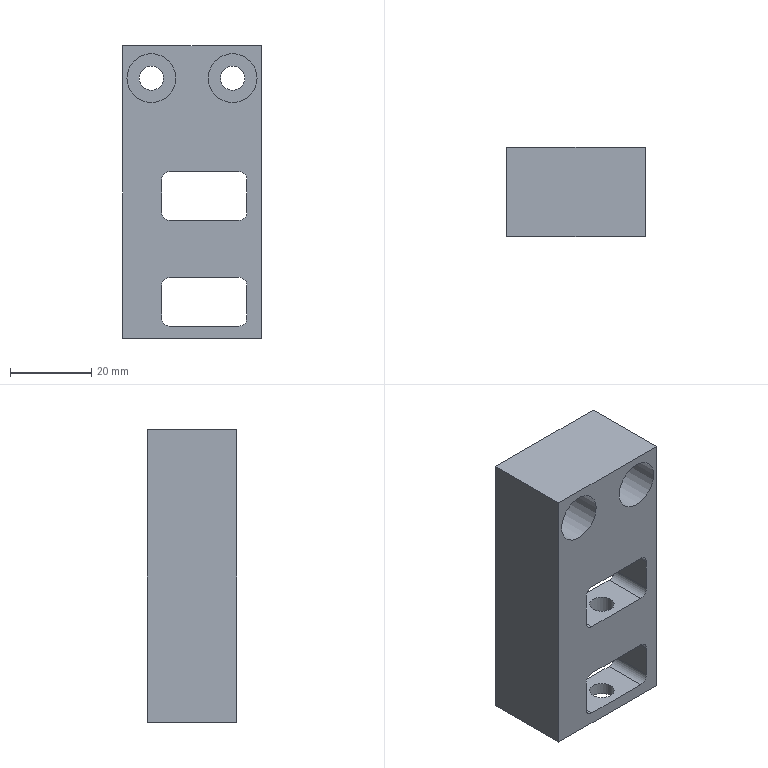Part | NX | features BREP 1, DATUM_CSYS 1 | 1 solid | 37 faces | volume 28457 mm3 | plane 19 | cylinder 17 | cone 1 | commonest cylinder face diameters 4 x8 6 x4 12 x3 5 x2